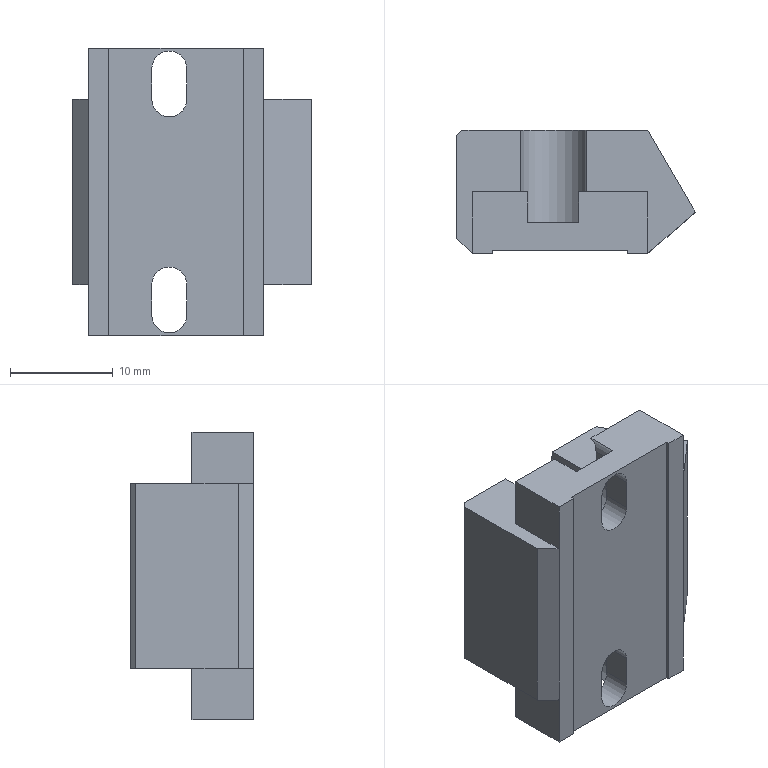Part | SolidWorks | features ICE 10, MoveFace 3, Chamfer 2, DelFace 2, Extrusion 1, HoleWzd 1 | 1 solid | 70 faces | box 23.18 x 12 x 28 mm | volume 4754 mm3 | plane 37 | cylinder 25 | cone 8 | commonest cylinder face diameters 1.6 x8 6.4 x7 3.4 x6 2 x4